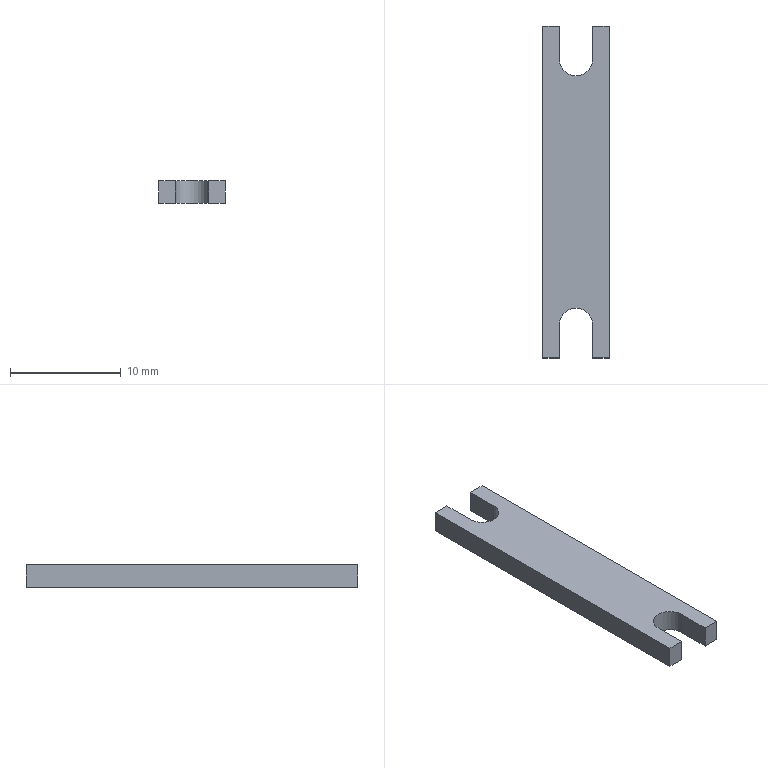Part | SolidWorks | features Extrusion 1 | 1 solid | 14 faces | box 6 x 30 x 2 mm | volume 309.863 mm3 | plane 12 | cylinder 2 | commonest cylinder face diameters 3 x2
STEP:
#1=CARTESIAN_POINT('',(3.,15.,0.));
#2=VERTEX_POINT('',#1);
#3=CARTESIAN_POINT('',(1.5,15.,0.));
#4=VERTEX_POINT('',#3);
#5=CARTESIAN_POINT('',(3.,15.,0.));
#6=DIRECTION('',(-1.,0.,0.));
#7=VECTOR('',#6,1000.);
#8=LINE('',#5,#7);
#9=EDGE_CURVE('',#2,#4,#8,.T.);
#10=ORIENTED_EDGE('',*,*,#9,.T.);
#11=CARTESIAN_POINT('',(1.5,15.,2.));
#12=VERTEX_POINT('',#11);
#13=CARTESIAN_POINT('',(1.5,15.,2.));
#14=DIRECTION('',(0.,0.,-1.));
#15=VECTOR('',#14,1000.);
#16=LINE('',#13,#15);
#17=EDGE_CURVE('',#12,#4,#16,.T.);
#18=ORIENTED_EDGE('',*,*,#17,.F.);
#19=CARTESIAN_POINT('',(3.,15.,2.));
#20=VERTEX_POINT('',#19);
#21=CARTESIAN_POINT('',(3.,15.,2.));
#22=DIRECTION('',(-1.,0.,0.));
#23=VECTOR('',#22,1000.);
#24=LINE('',#21,#23);
#25=EDGE_CURVE('',#20,#12,#24,.T.);
#26=ORIENTED_EDGE('',*,*,#25,.F.);
#27=CARTESIAN_POINT('',(3.,15.,2.));
#28=DIRECTION('',(0.,0.,-1.));
#29=VECTOR('',#28,1000.);
#30=LINE('',#27,#29);
#31=EDGE_CURVE('',#20,#2,#30,.T.);
#32=ORIENTED_EDGE('',*,*,#31,.T.);
#33=EDGE_LOOP('',(#10,#18,#26,#32));
#34=FACE_OUTER_BOUND('',#33,.T.);
#35=CARTESIAN_POINT('',(3.,15.,2.));
#36=DIRECTION('',(0.,-1.,0.));
#37=DIRECTION('',(0.,0.,-1.));
#38=AXIS2_PLACEMENT_3D('',#35,#36,#37);
#39=PLANE('',#38);
#40=ADVANCED_FACE('',(#34),#39,.F.);
#41=CARTESIAN_POINT('',(1.5,12.,0.));
#42=VERTEX_POINT('',#41);
#43=CARTESIAN_POINT('',(1.5,15.,0.));
#44=DIRECTION('',(0.,-1.,0.));
#45=VECTOR('',#44,1000.);
#46=LINE('',#43,#45);
#47=EDGE_CURVE('',#4,#42,#46,.T.);
#48=ORIENTED_EDGE('',*,*,#47,.T.);
#49=CARTESIAN_POINT('',(1.5,12.,2.));
#50=VERTEX_POINT('',#49);
#51=CARTESIAN_POINT('',(1.5,12.,2.));
#52=DIRECTION('',(0.,0.,-1.));
#53=VECTOR('',#52,1000.);
#54=LINE('',#51,#53);
#55=EDGE_CURVE('',#50,#42,#54,.T.);
#56=ORIENTED_EDGE('',*,*,#55,.F.);
#57=CARTESIAN_POINT('',(1.5,15.,2.));
#58=DIRECTION('',(0.,-1.,0.));
#59=VECTOR('',#58,1000.);
#60=LINE('',#57,#59);
#61=EDGE_CURVE('',#12,#50,#60,.T.);
#62=ORIENTED_EDGE('',*,*,#61,.F.);
#63=ORIENTED_EDGE('',*,*,#17,.T.);
#64=EDGE_LOOP('',(#48,#56,#62,#63));
#65=FACE_OUTER_BOUND('',#64,.T.);
#66=CARTESIAN_POINT('',(1.5,15.,2.));
#67=DIRECTION('',(1.,0.,0.));
#68=DIRECTION('',(0.,1.,0.));
#69=AXIS2_PLACEMENT_3D('',#66,#67,#68);
#70=PLANE('',#69);
#71=ADVANCED_FACE('',(#65),#70,.F.);
#72=CARTESIAN_POINT('',(-1.5,12.,0.));
#73=VERTEX_POINT('',#72);
#74=CARTESIAN_POINT('',(0.,12.,0.));
#75=DIRECTION('',(0.,0.,-1.));
#76=DIRECTION('',(1.,0.,0.));
#77=AXIS2_PLACEMENT_3D('',#74,#75,#76);
#78=CIRCLE('',#77,1.5);
#79=EDGE_CURVE('',#42,#73,#78,.T.);
#80=ORIENTED_EDGE('',*,*,#79,.T.);
#81=CARTESIAN_POINT('',(-1.5,12.,2.));
#82=VERTEX_POINT('',#81);
#83=CARTESIAN_POINT('',(-1.5,12.,2.));
#84=DIRECTION('',(0.,0.,-1.));
#85=VECTOR('',#84,1000.);
#86=LINE('',#83,#85);
#87=EDGE_CURVE('',#82,#73,#86,.T.);
#88=ORIENTED_EDGE('',*,*,#87,.F.);
#89=CARTESIAN_POINT('',(0.,12.,2.));
#90=DIRECTION('',(0.,0.,-1.));
#91=DIRECTION('',(1.,0.,0.));
#92=AXIS2_PLACEMENT_3D('',#89,#90,#91);
#93=CIRCLE('',#92,1.5);
#94=EDGE_CURVE('',#50,#82,#93,.T.);
#95=ORIENTED_EDGE('',*,*,#94,.F.);
#96=ORIENTED_EDGE('',*,*,#55,.T.);
#97=EDGE_LOOP('',(#80,#88,#95,#96));
#98=FACE_OUTER_BOUND('',#97,.T.);
#99=CARTESIAN_POINT('',(0.,12.,2.));
#100=DIRECTION('',(0.,0.,-1.));
#101=DIRECTION('',(-1.,0.,0.));
#102=AXIS2_PLACEMENT_3D('',#99,#100,#101);
#103=CYLINDRICAL_SURFACE('',#102,1.5);
#104=ADVANCED_FACE('',(#98),#103,.F.);
#105=CARTESIAN_POINT('',(-1.5,15.,0.));
#106=VERTEX_POINT('',#105);
#107=CARTESIAN_POINT('',(-1.5,15.,0.));
#108=DIRECTION('',(0.,1.,0.));
#109=VECTOR('',#108,1000.);
#110=LINE('',#107,#109);
#111=EDGE_CURVE('',#73,#106,#110,.T.);
#112=ORIENTED_EDGE('',*,*,#111,.T.);
#113=CARTESIAN_POINT('',(-1.5,15.,2.));
#114=VERTEX_POINT('',#113);
#115=CARTESIAN_POINT('',(-1.5,15.,2.));
#116=DIRECTION('',(0.,0.,-1.));
#117=VECTOR('',#116,1000.);
#118=LINE('',#115,#117);
#119=EDGE_CURVE('',#114,#106,#118,.T.);
#120=ORIENTED_EDGE('',*,*,#119,.F.);
#121=CARTESIAN_POINT('',(-1.5,15.,2.));
#122=DIRECTION('',(0.,1.,0.));
#123=VECTOR('',#122,1000.);
#124=LINE('',#121,#123);
#125=EDGE_CURVE('',#82,#114,#124,.T.);
#126=ORIENTED_EDGE('',*,*,#125,.F.);
#127=ORIENTED_EDGE('',*,*,#87,.T.);
#128=EDGE_LOOP('',(#112,#120,#126,#127));
#129=FACE_OUTER_BOUND('',#128,.T.);
#130=CARTESIAN_POINT('',(-1.5,15.,2.));
#131=DIRECTION('',(-1.,0.,0.));
#132=DIRECTION('',(0.,-1.,0.));
#133=AXIS2_PLACEMENT_3D('',#130,#131,#132);
#134=PLANE('',#133);
#135=ADVANCED_FACE('',(#129),#134,.F.);
#136=CARTESIAN_POINT('',(-3.,15.,0.));
#137=VERTEX_POINT('',#136);
#138=CARTESIAN_POINT('',(-3.,15.,0.));
#139=DIRECTION('',(-1.,0.,0.));
#140=VECTOR('',#139,1000.);
#141=LINE('',#138,#140);
#142=EDGE_CURVE('',#106,#137,#141,.T.);
#143=ORIENTED_EDGE('',*,*,#142,.T.);
#144=CARTESIAN_POINT('',(-3.,15.,2.));
#145=VERTEX_POINT('',#144);
#146=CARTESIAN_POINT('',(-3.,15.,2.));
#147=DIRECTION('',(0.,0.,-1.));
#148=VECTOR('',#147,1000.);
#149=LINE('',#146,#148);
#150=EDGE_CURVE('',#145,#137,#149,.T.);
#151=ORIENTED_EDGE('',*,*,#150,.F.);
#152=CARTESIAN_POINT('',(-3.,15.,2.));
#153=DIRECTION('',(-1.,0.,0.));
#154=VECTOR('',#153,1000.);
#155=LINE('',#152,#154);
#156=EDGE_CURVE('',#114,#145,#155,.T.);
#157=ORIENTED_EDGE('',*,*,#156,.F.);
#158=ORIENTED_EDGE('',*,*,#119,.T.);
#159=EDGE_LOOP('',(#143,#151,#157,#158));
#160=FACE_OUTER_BOUND('',#159,.T.);
#161=CARTESIAN_POINT('',(-3.,15.,2.));
#162=DIRECTION('',(0.,-1.,0.));
#163=DIRECTION('',(0.,0.,-1.));
#164=AXIS2_PLACEMENT_3D('',#161,#162,#163);
#165=PLANE('',#164);
#166=ADVANCED_FACE('',(#160),#165,.F.);
#167=CARTESIAN_POINT('',(-3.,-15.,0.));
#168=VERTEX_POINT('',#167);
#169=CARTESIAN_POINT('',(-3.,15.,0.));
#170=DIRECTION('',(0.,-1.,0.));
#171=VECTOR('',#170,1000.);
#172=LINE('',#169,#171);
#173=EDGE_CURVE('',#137,#168,#172,.T.);
#174=ORIENTED_EDGE('',*,*,#173,.T.);
#175=CARTESIAN_POINT('',(-3.,-15.,2.));
#176=VERTEX_POINT('',#175);
#177=CARTESIAN_POINT('',(-3.,-15.,2.));
#178=DIRECTION('',(0.,0.,-1.));
#179=VECTOR('',#178,1000.);
#180=LINE('',#177,#179);
#181=EDGE_CURVE('',#176,#168,#180,.T.);
#182=ORIENTED_EDGE('',*,*,#181,.F.);
#183=CARTESIAN_POINT('',(-3.,15.,2.));
#184=DIRECTION('',(0.,-1.,0.));
#185=VECTOR('',#184,1000.);
#186=LINE('',#183,#185);
#187=EDGE_CURVE('',#145,#176,#186,.T.);
#188=ORIENTED_EDGE('',*,*,#187,.F.);
#189=ORIENTED_EDGE('',*,*,#150,.T.);
#190=EDGE_LOOP('',(#174,#182,#188,#189));
#191=FACE_OUTER_BOUND('',#190,.T.);
#192=CARTESIAN_POINT('',(-3.,15.,2.));
#193=DIRECTION('',(1.,0.,0.));
#194=DIRECTION('',(0.,1.,0.));
#195=AXIS2_PLACEMENT_3D('',#192,#193,#194);
#196=PLANE('',#195);
#197=ADVANCED_FACE('',(#191),#196,.F.);
#198=CARTESIAN_POINT('',(-1.5,-15.,0.));
#199=VERTEX_POINT('',#198);
#200=CARTESIAN_POINT('',(-3.,-15.,0.));
#201=DIRECTION('',(1.,0.,0.));
#202=VECTOR('',#201,1000.);
#203=LINE('',#200,#202);
#204=EDGE_CURVE('',#168,#199,#203,.T.);
#205=ORIENTED_EDGE('',*,*,#204,.T.);
#206=CARTESIAN_POINT('',(-1.5,-15.,2.));
#207=VERTEX_POINT('',#206);
#208=CARTESIAN_POINT('',(-1.5,-15.,2.));
#209=DIRECTION('',(0.,0.,-1.));
#210=VECTOR('',#209,1000.);
#211=LINE('',#208,#210);
#212=EDGE_CURVE('',#207,#199,#211,.T.);
#213=ORIENTED_EDGE('',*,*,#212,.F.);
#214=CARTESIAN_POINT('',(-3.,-15.,2.));
#215=DIRECTION('',(1.,0.,0.));
#216=VECTOR('',#215,1000.);
#217=LINE('',#214,#216);
#218=EDGE_CURVE('',#176,#207,#217,.T.);
#219=ORIENTED_EDGE('',*,*,#218,.F.);
#220=ORIENTED_EDGE('',*,*,#181,.T.);
#221=EDGE_LOOP('',(#205,#213,#219,#220));
#222=FACE_OUTER_BOUND('',#221,.T.);
#223=CARTESIAN_POINT('',(-3.,-15.,2.));
#224=DIRECTION('',(0.,1.,0.));
#225=DIRECTION('',(0.,0.,1.));
#226=AXIS2_PLACEMENT_3D('',#223,#224,#225);
#227=PLANE('',#226);
#228=ADVANCED_FACE('',(#222),#227,.F.);
#229=CARTESIAN_POINT('',(-1.5,-12.,0.));
#230=VERTEX_POINT('',#229);
#231=CARTESIAN_POINT('',(-1.5,-15.,0.));
#232=DIRECTION('',(0.,1.,0.));
#233=VECTOR('',#232,1000.);
#234=LINE('',#231,#233);
#235=EDGE_CURVE('',#199,#230,#234,.T.);
#236=ORIENTED_EDGE('',*,*,#235,.T.);
#237=CARTESIAN_POINT('',(-1.5,-12.,2.));
#238=VERTEX_POINT('',#237);
#239=CARTESIAN_POINT('',(-1.5,-12.,2.));
#240=DIRECTION('',(0.,0.,-1.));
#241=VECTOR('',#240,1000.);
#242=LINE('',#239,#241);
#243=EDGE_CURVE('',#238,#230,#242,.T.);
#244=ORIENTED_EDGE('',*,*,#243,.F.);
#245=CARTESIAN_POINT('',(-1.5,-15.,2.));
#246=DIRECTION('',(0.,1.,0.));
#247=VECTOR('',#246,1000.);
#248=LINE('',#245,#247);
#249=EDGE_CURVE('',#207,#238,#248,.T.);
#250=ORIENTED_EDGE('',*,*,#249,.F.);
#251=ORIENTED_EDGE('',*,*,#212,.T.);
#252=EDGE_LOOP('',(#236,#244,#250,#251));
#253=FACE_OUTER_BOUND('',#252,.T.);
#254=CARTESIAN_POINT('',(-1.5,-15.,2.));
#255=DIRECTION('',(-1.,0.,0.));
#256=DIRECTION('',(0.,-1.,0.));
#257=AXIS2_PLACEMENT_3D('',#254,#255,#256);
#258=PLANE('',#257);
#259=ADVANCED_FACE('',(#253),#258,.F.);
#260=CARTESIAN_POINT('',(1.5,-12.,0.));
#261=VERTEX_POINT('',#260);
#262=CARTESIAN_POINT('',(0.,-12.,0.));
#263=DIRECTION('',(0.,0.,-1.));
#264=DIRECTION('',(1.,0.,0.));
#265=AXIS2_PLACEMENT_3D('',#262,#263,#264);
#266=CIRCLE('',#265,1.5);
#267=EDGE_CURVE('',#230,#261,#266,.T.);
#268=ORIENTED_EDGE('',*,*,#267,.T.);
#269=CARTESIAN_POINT('',(1.5,-12.,2.));
#270=VERTEX_POINT('',#269);
#271=CARTESIAN_POINT('',(1.5,-12.,2.));
#272=DIRECTION('',(0.,0.,-1.));
#273=VECTOR('',#272,1000.);
#274=LINE('',#271,#273);
#275=EDGE_CURVE('',#270,#261,#274,.T.);
#276=ORIENTED_EDGE('',*,*,#275,.F.);
#277=CARTESIAN_POINT('',(0.,-12.,2.));
#278=DIRECTION('',(0.,0.,-1.));
#279=DIRECTION('',(1.,0.,0.));
#280=AXIS2_PLACEMENT_3D('',#277,#278,#279);
#281=CIRCLE('',#280,1.5);
#282=EDGE_CURVE('',#238,#270,#281,.T.);
#283=ORIENTED_EDGE('',*,*,#282,.F.);
#284=ORIENTED_EDGE('',*,*,#243,.T.);
#285=EDGE_LOOP('',(#268,#276,#283,#284));
#286=FACE_OUTER_BOUND('',#285,.T.);
#287=CARTESIAN_POINT('',(0.,-12.,2.));
#288=DIRECTION('',(0.,0.,-1.));
#289=DIRECTION('',(-1.,0.,0.));
#290=AXIS2_PLACEMENT_3D('',#287,#288,#289);
#291=CYLINDRICAL_SURFACE('',#290,1.5);
#292=ADVANCED_FACE('',(#286),#291,.F.);
#293=CARTESIAN_POINT('',(1.5,-15.,0.));
#294=VERTEX_POINT('',#293);
#295=CARTESIAN_POINT('',(1.5,-15.,0.));
#296=DIRECTION('',(0.,-1.,0.));
#297=VECTOR('',#296,1000.);
#298=LINE('',#295,#297);
#299=EDGE_CURVE('',#261,#294,#298,.T.);
#300=ORIENTED_EDGE('',*,*,#299,.T.);
#301=CARTESIAN_POINT('',(1.5,-15.,2.));
#302=VERTEX_POINT('',#301);
#303=CARTESIAN_POINT('',(1.5,-15.,2.));
#304=DIRECTION('',(0.,0.,-1.));
#305=VECTOR('',#304,1000.);
#306=LINE('',#303,#305);
#307=EDGE_CURVE('',#302,#294,#306,.T.);
#308=ORIENTED_EDGE('',*,*,#307,.F.);
#309=CARTESIAN_POINT('',(1.5,-15.,2.));
#310=DIRECTION('',(0.,-1.,0.));
#311=VECTOR('',#310,1000.);
#312=LINE('',#309,#311);
#313=EDGE_CURVE('',#270,#302,#312,.T.);
#314=ORIENTED_EDGE('',*,*,#313,.F.);
#315=ORIENTED_EDGE('',*,*,#275,.T.);
#316=EDGE_LOOP('',(#300,#308,#314,#315));
#317=FACE_OUTER_BOUND('',#316,.T.);
#318=CARTESIAN_POINT('',(1.5,-15.,2.));
#319=DIRECTION('',(1.,0.,0.));
#320=DIRECTION('',(0.,1.,0.));
#321=AXIS2_PLACEMENT_3D('',#318,#319,#320);
#322=PLANE('',#321);
#323=ADVANCED_FACE('',(#317),#322,.F.);
#324=CARTESIAN_POINT('',(3.,-15.,0.));
#325=VERTEX_POINT('',#324);
#326=CARTESIAN_POINT('',(3.,-15.,0.));
#327=DIRECTION('',(1.,0.,0.));
#328=VECTOR('',#327,1000.);
#329=LINE('',#326,#328);
#330=EDGE_CURVE('',#294,#325,#329,.T.);
#331=ORIENTED_EDGE('',*,*,#330,.T.);
#332=CARTESIAN_POINT('',(3.,-15.,2.));
#333=VERTEX_POINT('',#332);
#334=CARTESIAN_POINT('',(3.,-15.,2.));
#335=DIRECTION('',(0.,0.,-1.));
#336=VECTOR('',#335,1000.);
#337=LINE('',#334,#336);
#338=EDGE_CURVE('',#333,#325,#337,.T.);
#339=ORIENTED_EDGE('',*,*,#338,.F.);
#340=CARTESIAN_POINT('',(3.,-15.,2.));
#341=DIRECTION('',(1.,0.,0.));
#342=VECTOR('',#341,1000.);
#343=LINE('',#340,#342);
#344=EDGE_CURVE('',#302,#333,#343,.T.);
#345=ORIENTED_EDGE('',*,*,#344,.F.);
#346=ORIENTED_EDGE('',*,*,#307,.T.);
#347=EDGE_LOOP('',(#331,#339,#345,#346));
#348=FACE_OUTER_BOUND('',#347,.T.);
#349=CARTESIAN_POINT('',(3.,-15.,2.));
#350=DIRECTION('',(0.,1.,0.));
#351=DIRECTION('',(0.,0.,1.));
#352=AXIS2_PLACEMENT_3D('',#349,#350,#351);
#353=PLANE('',#352);
#354=ADVANCED_FACE('',(#348),#353,.F.);
#355=CARTESIAN_POINT('',(3.,15.,0.));
#356=DIRECTION('',(0.,1.,0.));
#357=VECTOR('',#356,1000.);
#358=LINE('',#355,#357);
#359=EDGE_CURVE('',#325,#2,#358,.T.);
#360=ORIENTED_EDGE('',*,*,#359,.T.);
#361=ORIENTED_EDGE('',*,*,#31,.F.);
#362=CARTESIAN_POINT('',(3.,15.,2.));
#363=DIRECTION('',(0.,1.,0.));
#364=VECTOR('',#363,1000.);
#365=LINE('',#362,#364);
#366=EDGE_CURVE('',#333,#20,#365,.T.);
#367=ORIENTED_EDGE('',*,*,#366,.F.);
#368=ORIENTED_EDGE('',*,*,#338,.T.);
#369=EDGE_LOOP('',(#360,#361,#367,#368));
#370=FACE_OUTER_BOUND('',#369,.T.);
#371=CARTESIAN_POINT('',(3.,15.,2.));
#372=DIRECTION('',(-1.,0.,0.));
#373=DIRECTION('',(0.,-1.,0.));
#374=AXIS2_PLACEMENT_3D('',#371,#372,#373);
#375=PLANE('',#374);
#376=ADVANCED_FACE('',(#370),#375,.F.);
#377=ORIENTED_EDGE('',*,*,#25,.T.);
#378=ORIENTED_EDGE('',*,*,#61,.T.);
#379=ORIENTED_EDGE('',*,*,#94,.T.);
#380=ORIENTED_EDGE('',*,*,#125,.T.);
#381=ORIENTED_EDGE('',*,*,#156,.T.);
#382=ORIENTED_EDGE('',*,*,#187,.T.);
#383=ORIENTED_EDGE('',*,*,#218,.T.);
#384=ORIENTED_EDGE('',*,*,#249,.T.);
#385=ORIENTED_EDGE('',*,*,#282,.T.);
#386=ORIENTED_EDGE('',*,*,#313,.T.);
#387=ORIENTED_EDGE('',*,*,#344,.T.);
#388=ORIENTED_EDGE('',*,*,#366,.T.);
#389=EDGE_LOOP('',(#377,#378,#379,#380,#381,#382,#383,#384,#385,#386,#387,#388));
#390=FACE_OUTER_BOUND('',#389,.T.);
#391=CARTESIAN_POINT('',(0.,12.,2.));
#392=DIRECTION('',(0.,0.,1.));
#393=DIRECTION('',(1.,0.,0.));
#394=AXIS2_PLACEMENT_3D('',#391,#392,#393);
#395=PLANE('',#394);
#396=ADVANCED_FACE('',(#390),#395,.T.);
#397=ORIENTED_EDGE('',*,*,#9,.F.);
#398=ORIENTED_EDGE('',*,*,#359,.F.);
#399=ORIENTED_EDGE('',*,*,#330,.F.);
#400=ORIENTED_EDGE('',*,*,#299,.F.);
#401=ORIENTED_EDGE('',*,*,#267,.F.);
#402=ORIENTED_EDGE('',*,*,#235,.F.);
#403=ORIENTED_EDGE('',*,*,#204,.F.);
#404=ORIENTED_EDGE('',*,*,#173,.F.);
#405=ORIENTED_EDGE('',*,*,#142,.F.);
#406=ORIENTED_EDGE('',*,*,#111,.F.);
#407=ORIENTED_EDGE('',*,*,#79,.F.);
#408=ORIENTED_EDGE('',*,*,#47,.F.);
#409=EDGE_LOOP('',(#397,#398,#399,#400,#401,#402,#403,#404,#405,#406,#407,#408));
#410=FACE_OUTER_BOUND('',#409,.T.);
#411=CARTESIAN_POINT('',(0.,12.,0.));
#412=DIRECTION('',(0.,0.,1.));
#413=DIRECTION('',(1.,0.,0.));
#414=AXIS2_PLACEMENT_3D('',#411,#412,#413);
#415=PLANE('',#414);
#416=ADVANCED_FACE('',(#410),#415,.F.);
#417=CLOSED_SHELL('',(#40,#71,#104,#135,#166,#197,#228,#259,#292,#323,#354,#376,#396,#416));
#418=MANIFOLD_SOLID_BREP('',#417);
#419=CARTESIAN_POINT('',(0.,0.,0.));
#420=DIRECTION('',(0.,0.,1.));
#421=DIRECTION('',(1.,0.,0.));
#422=AXIS2_PLACEMENT_3D('',#419,#420,#421);
#423=(LENGTH_UNIT()NAMED_UNIT(*)SI_UNIT(.MILLI.,.METRE.));
#424=UNCERTAINTY_MEASURE_WITH_UNIT(LENGTH_MEASURE(0.00001),#423,'','');
#425=(NAMED_UNIT(*)PLANE_ANGLE_UNIT()SI_UNIT($,.RADIAN.));
#426=(NAMED_UNIT(*)SI_UNIT($,.STERADIAN.)SOLID_ANGLE_UNIT());
#427=(GEOMETRIC_REPRESENTATION_CONTEXT(3)GLOBAL_UNCERTAINTY_ASSIGNED_CONTEXT((#424))GLOBAL_UNIT_ASSIGNED_CONTEXT((#423,#425,#426))REPRESENTATION_CONTEXT('',''));
#428=ADVANCED_BREP_SHAPE_REPRESENTATION('',(#418,#422),#427);